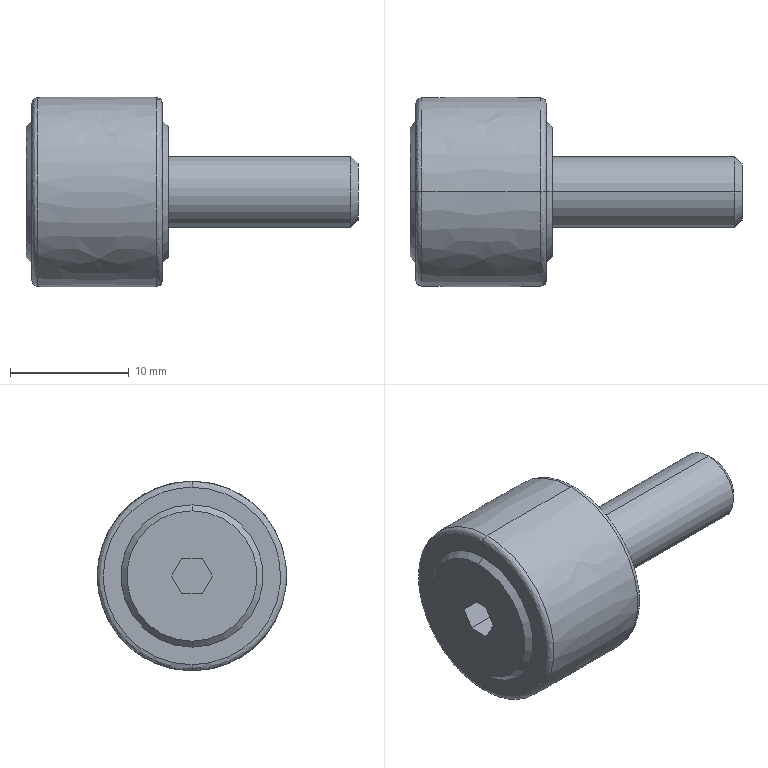Part | STEP file | 0229_Z_CFUA6-16_1 | 1 solid | 26 faces | box 28 x 15.999 x 16 mm | volume 2735 mm3 | plane 12 | spline 6 | cone 6 | cylinder 2 | commonest cylinder face diameters 6 x2